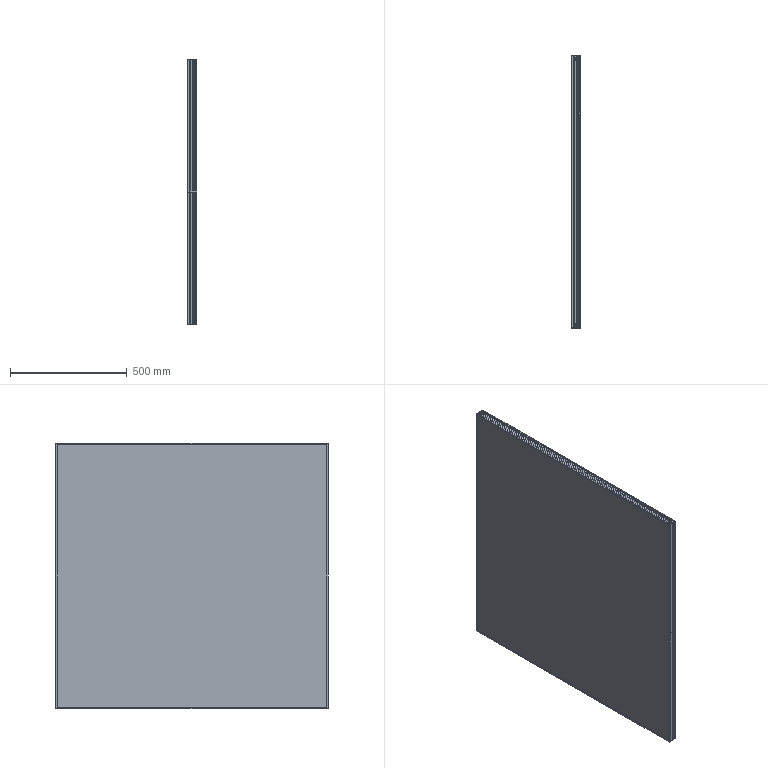Part | 7 solids | 390 faces | box 40 x 1170 x 1140 mm | volume 15853080 mm3 | plane 254 | cylinder 136 | commonest cylinder face diameters 0.6 x80 4 x32 3 x16 5 x8